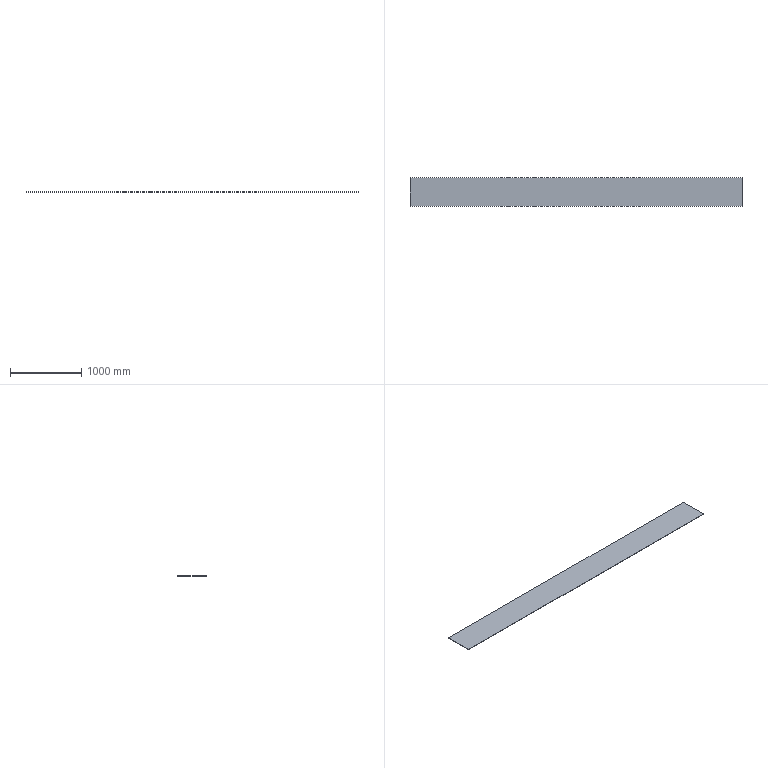Part | SolidWorks | features FlatPattern 1, SMBaseFlange 1, SheetMetal 1 | 1 solid | 6 faces | box 4660 x 400 x 5 mm | volume 9320000 mm3 | plane 6
STEP:
#1=CARTESIAN_POINT('',(0.,400.,0.));
#2=VERTEX_POINT('',#1);
#3=CARTESIAN_POINT('',(0.,0.,0.));
#4=VERTEX_POINT('',#3);
#5=CARTESIAN_POINT('',(0.,0.,0.));
#6=DIRECTION('',(0.,-1.,0.));
#7=VECTOR('',#6,1000.);
#8=LINE('',#5,#7);
#9=EDGE_CURVE('',#2,#4,#8,.T.);
#10=ORIENTED_EDGE('',*,*,#9,.F.);
#11=CARTESIAN_POINT('',(0.,400.,-5.));
#12=VERTEX_POINT('',#11);
#13=CARTESIAN_POINT('',(0.,400.,-5.));
#14=DIRECTION('',(0.,0.,1.));
#15=VECTOR('',#14,1000.);
#16=LINE('',#13,#15);
#17=EDGE_CURVE('',#12,#2,#16,.T.);
#18=ORIENTED_EDGE('',*,*,#17,.F.);
#19=CARTESIAN_POINT('',(0.,0.,-5.));
#20=VERTEX_POINT('',#19);
#21=CARTESIAN_POINT('',(0.,0.,-5.));
#22=DIRECTION('',(0.,-1.,0.));
#23=VECTOR('',#22,1000.);
#24=LINE('',#21,#23);
#25=EDGE_CURVE('',#12,#20,#24,.T.);
#26=ORIENTED_EDGE('',*,*,#25,.T.);
#27=CARTESIAN_POINT('',(0.,0.,-5.));
#28=DIRECTION('',(0.,0.,1.));
#29=VECTOR('',#28,1000.);
#30=LINE('',#27,#29);
#31=EDGE_CURVE('',#20,#4,#30,.T.);
#32=ORIENTED_EDGE('',*,*,#31,.T.);
#33=EDGE_LOOP('',(#10,#18,#26,#32));
#34=FACE_OUTER_BOUND('',#33,.T.);
#35=CARTESIAN_POINT('',(0.,0.,-5.));
#36=DIRECTION('',(-1.,0.,0.));
#37=DIRECTION('',(0.,0.,1.));
#38=AXIS2_PLACEMENT_3D('',#35,#36,#37);
#39=PLANE('',#38);
#40=ADVANCED_FACE('',(#34),#39,.T.);
#41=CARTESIAN_POINT('',(4660.,400.,0.));
#42=VERTEX_POINT('',#41);
#43=CARTESIAN_POINT('',(0.,400.,0.));
#44=DIRECTION('',(-1.,0.,0.));
#45=VECTOR('',#44,1000.);
#46=LINE('',#43,#45);
#47=EDGE_CURVE('',#42,#2,#46,.T.);
#48=ORIENTED_EDGE('',*,*,#47,.F.);
#49=CARTESIAN_POINT('',(4660.,400.,-5.));
#50=VERTEX_POINT('',#49);
#51=CARTESIAN_POINT('',(4660.,400.,-5.));
#52=DIRECTION('',(0.,0.,1.));
#53=VECTOR('',#52,1000.);
#54=LINE('',#51,#53);
#55=EDGE_CURVE('',#50,#42,#54,.T.);
#56=ORIENTED_EDGE('',*,*,#55,.F.);
#57=CARTESIAN_POINT('',(0.,400.,-5.));
#58=DIRECTION('',(-1.,0.,0.));
#59=VECTOR('',#58,1000.);
#60=LINE('',#57,#59);
#61=EDGE_CURVE('',#50,#12,#60,.T.);
#62=ORIENTED_EDGE('',*,*,#61,.T.);
#63=ORIENTED_EDGE('',*,*,#17,.T.);
#64=EDGE_LOOP('',(#48,#56,#62,#63));
#65=FACE_OUTER_BOUND('',#64,.T.);
#66=CARTESIAN_POINT('',(0.,400.,-5.));
#67=DIRECTION('',(0.,1.,0.));
#68=DIRECTION('',(0.,0.,1.));
#69=AXIS2_PLACEMENT_3D('',#66,#67,#68);
#70=PLANE('',#69);
#71=ADVANCED_FACE('',(#65),#70,.T.);
#72=CARTESIAN_POINT('',(4660.,0.,0.));
#73=VERTEX_POINT('',#72);
#74=CARTESIAN_POINT('',(4660.,0.,0.));
#75=DIRECTION('',(0.,1.,0.));
#76=VECTOR('',#75,1000.);
#77=LINE('',#74,#76);
#78=EDGE_CURVE('',#73,#42,#77,.T.);
#79=ORIENTED_EDGE('',*,*,#78,.F.);
#80=CARTESIAN_POINT('',(4660.,0.,-5.));
#81=VERTEX_POINT('',#80);
#82=CARTESIAN_POINT('',(4660.,0.,-5.));
#83=DIRECTION('',(0.,0.,1.));
#84=VECTOR('',#83,1000.);
#85=LINE('',#82,#84);
#86=EDGE_CURVE('',#81,#73,#85,.T.);
#87=ORIENTED_EDGE('',*,*,#86,.F.);
#88=CARTESIAN_POINT('',(4660.,0.,-5.));
#89=DIRECTION('',(0.,1.,0.));
#90=VECTOR('',#89,1000.);
#91=LINE('',#88,#90);
#92=EDGE_CURVE('',#81,#50,#91,.T.);
#93=ORIENTED_EDGE('',*,*,#92,.T.);
#94=ORIENTED_EDGE('',*,*,#55,.T.);
#95=EDGE_LOOP('',(#79,#87,#93,#94));
#96=FACE_OUTER_BOUND('',#95,.T.);
#97=CARTESIAN_POINT('',(4660.,0.,-5.));
#98=DIRECTION('',(1.,0.,0.));
#99=DIRECTION('',(0.,0.,-1.));
#100=AXIS2_PLACEMENT_3D('',#97,#98,#99);
#101=PLANE('',#100);
#102=ADVANCED_FACE('',(#96),#101,.T.);
#103=CARTESIAN_POINT('',(0.,0.,0.));
#104=DIRECTION('',(1.,0.,0.));
#105=VECTOR('',#104,1000.);
#106=LINE('',#103,#105);
#107=EDGE_CURVE('',#4,#73,#106,.T.);
#108=ORIENTED_EDGE('',*,*,#107,.F.);
#109=ORIENTED_EDGE('',*,*,#31,.F.);
#110=CARTESIAN_POINT('',(0.,0.,-5.));
#111=DIRECTION('',(1.,0.,0.));
#112=VECTOR('',#111,1000.);
#113=LINE('',#110,#112);
#114=EDGE_CURVE('',#20,#81,#113,.T.);
#115=ORIENTED_EDGE('',*,*,#114,.T.);
#116=ORIENTED_EDGE('',*,*,#86,.T.);
#117=EDGE_LOOP('',(#108,#109,#115,#116));
#118=FACE_OUTER_BOUND('',#117,.T.);
#119=CARTESIAN_POINT('',(0.,0.,-5.));
#120=DIRECTION('',(0.,-1.,0.));
#121=DIRECTION('',(0.,0.,-1.));
#122=AXIS2_PLACEMENT_3D('',#119,#120,#121);
#123=PLANE('',#122);
#124=ADVANCED_FACE('',(#118),#123,.T.);
#125=ORIENTED_EDGE('',*,*,#25,.F.);
#126=ORIENTED_EDGE('',*,*,#61,.F.);
#127=ORIENTED_EDGE('',*,*,#92,.F.);
#128=ORIENTED_EDGE('',*,*,#114,.F.);
#129=EDGE_LOOP('',(#125,#126,#127,#128));
#130=FACE_OUTER_BOUND('',#129,.T.);
#131=CARTESIAN_POINT('',(0.,0.,-5.));
#132=DIRECTION('',(0.,0.,-1.));
#133=DIRECTION('',(-1.,0.,0.));
#134=AXIS2_PLACEMENT_3D('',#131,#132,#133);
#135=PLANE('',#134);
#136=ADVANCED_FACE('',(#130),#135,.T.);
#137=ORIENTED_EDGE('',*,*,#9,.T.);
#138=ORIENTED_EDGE('',*,*,#107,.T.);
#139=ORIENTED_EDGE('',*,*,#78,.T.);
#140=ORIENTED_EDGE('',*,*,#47,.T.);
#141=EDGE_LOOP('',(#137,#138,#139,#140));
#142=FACE_OUTER_BOUND('',#141,.T.);
#143=CARTESIAN_POINT('',(0.,0.,0.));
#144=DIRECTION('',(0.,0.,-1.));
#145=DIRECTION('',(-1.,0.,0.));
#146=AXIS2_PLACEMENT_3D('',#143,#144,#145);
#147=PLANE('',#146);
#148=ADVANCED_FACE('',(#142),#147,.F.);
#149=CLOSED_SHELL('',(#40,#71,#102,#124,#136,#148));
#150=MANIFOLD_SOLID_BREP('',#149);
#151=CARTESIAN_POINT('',(0.,0.,0.));
#152=DIRECTION('',(0.,0.,1.));
#153=DIRECTION('',(1.,0.,0.));
#154=AXIS2_PLACEMENT_3D('',#151,#152,#153);
#155=(LENGTH_UNIT()NAMED_UNIT(*)SI_UNIT(.MILLI.,.METRE.));
#156=UNCERTAINTY_MEASURE_WITH_UNIT(LENGTH_MEASURE(0.00001),#155,'','');
#157=(NAMED_UNIT(*)PLANE_ANGLE_UNIT()SI_UNIT($,.RADIAN.));
#158=(NAMED_UNIT(*)SI_UNIT($,.STERADIAN.)SOLID_ANGLE_UNIT());
#159=(GEOMETRIC_REPRESENTATION_CONTEXT(3)GLOBAL_UNCERTAINTY_ASSIGNED_CONTEXT((#156))GLOBAL_UNIT_ASSIGNED_CONTEXT((#155,#157,#158))REPRESENTATION_CONTEXT('',''));
#160=ADVANCED_BREP_SHAPE_REPRESENTATION('',(#150,#154),#159);